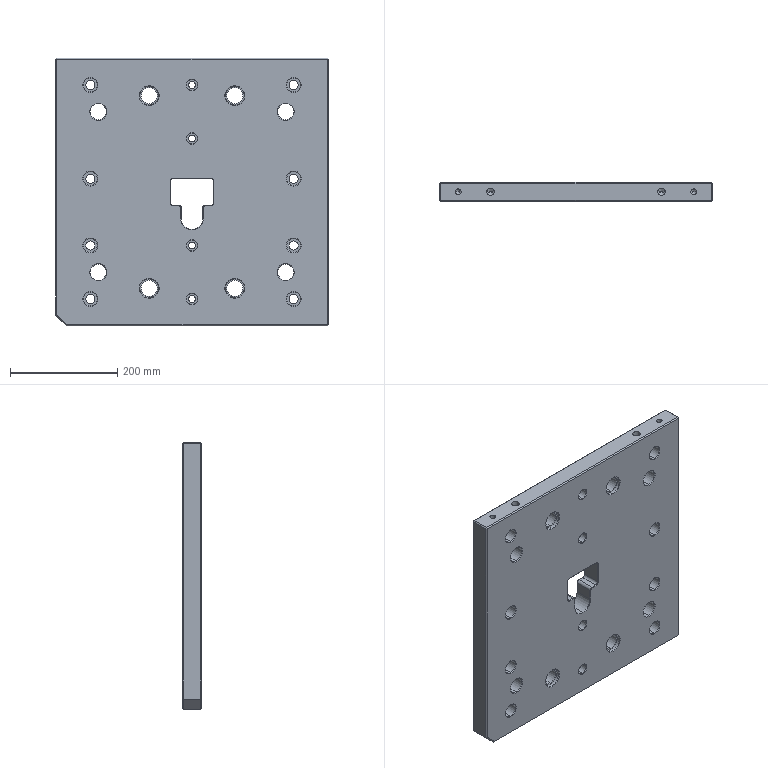Part | STEP file | PBI - 1 cav | 1 solid | 270 faces | box 510 x 36 x 500 mm | volume 8558348 mm3 | cone 111 | cylinder 96 | plane 63 | commonest cylinder face diameters 17 x16 26 x16 30 x16 10.5 x8 13 x8 14 x8